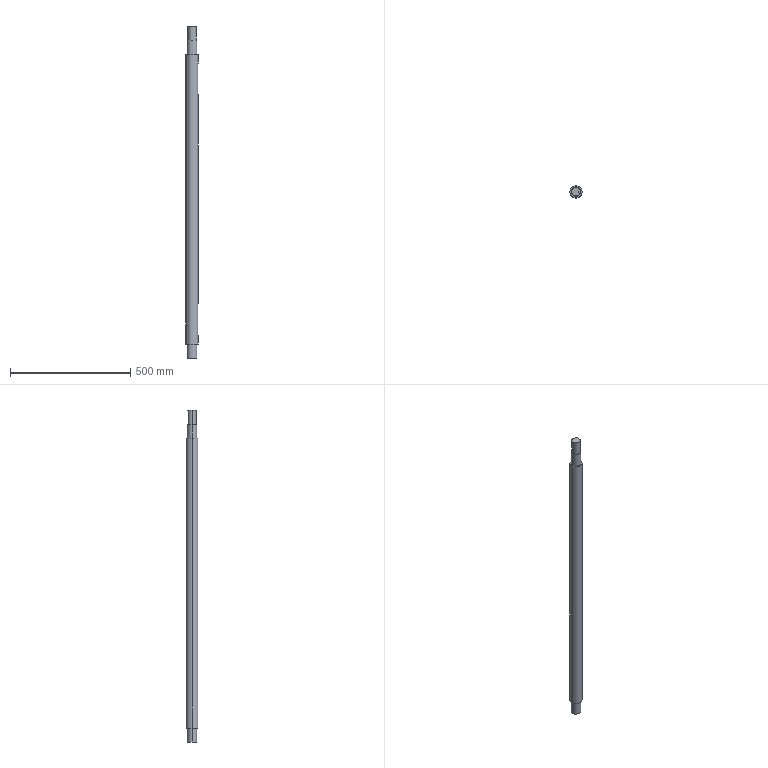Part | STEP file | Drive double sprocket shaft 1XG | 1 solid | 31 faces | box 50 x 50 x 1380 mm | volume 2550231 mm3 | cylinder 17 | plane 14 | commonest cylinder face diameters 12 x6 40 x4 10 x3 35 x2 50 x2